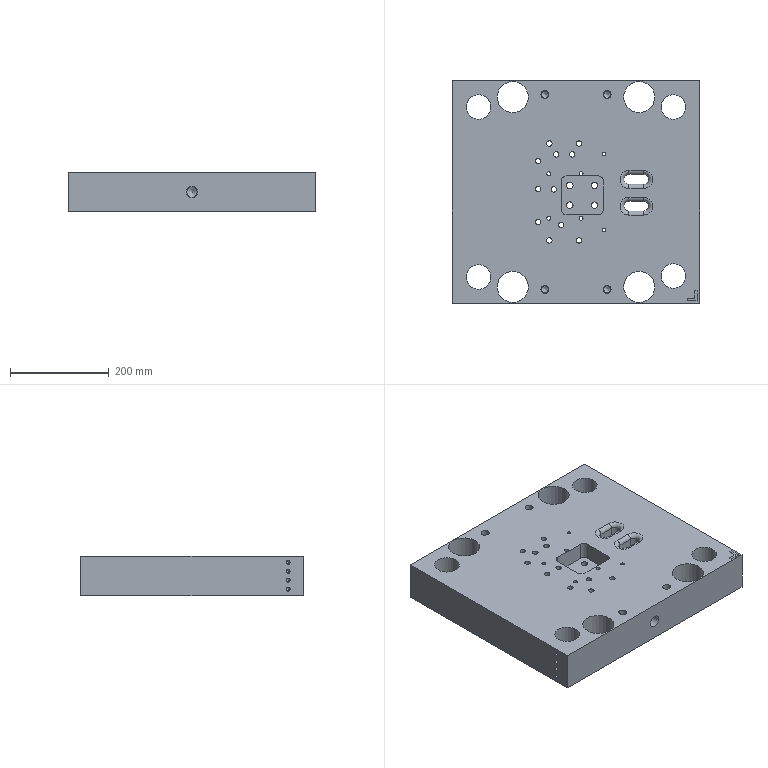Part | STEP file | BDB | 1 solid | 179 faces | box 500 x 450 x 80 mm | volume 15672052 mm3 | cylinder 97 | plane 50 | cone 24 | torus 8 | commonest cylinder face diameters 16 x18 8 x12 20 x12 11 x11 6.7 x8 15 x6